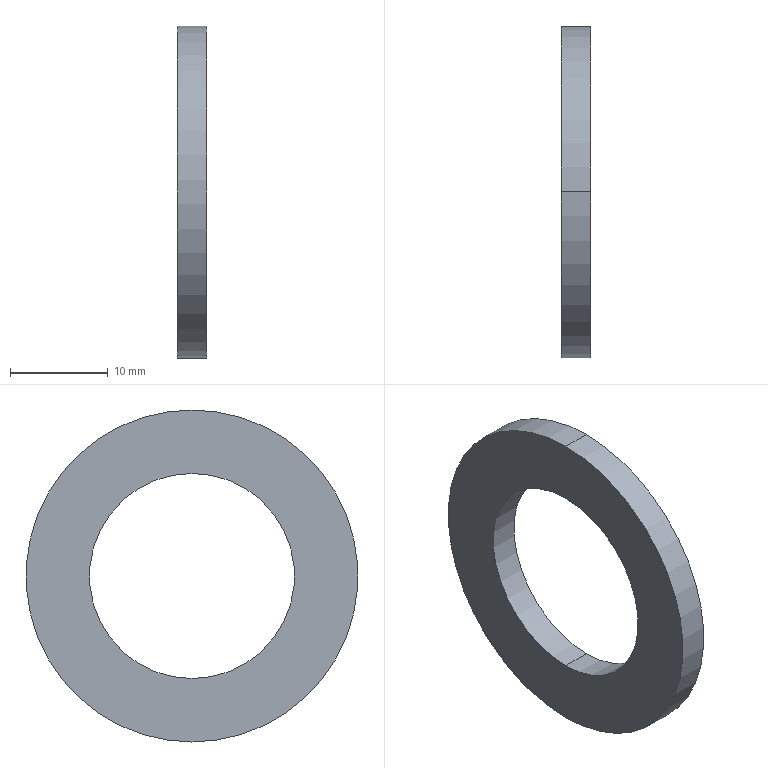Part | STEP file | plain washer small grade a_iso(Washer ISO 7092 - 20) | 1 solid | 6 faces | box 3 x 34 x 34 mm | volume 1685 mm3 | cylinder 4 | plane 2 | commonest cylinder face diameters 21 x2 34 x2
STEP:
#1=CARTESIAN_POINT('',(0.,0.,0.));
#2=DIRECTION('',(0.,0.,1.));
#3=DIRECTION('',(1.,0.,0.));
#4=AXIS2_PLACEMENT_3D('',#1,#2,#3);
#5=CARTESIAN_POINT('',(0.,0.,17.));
#6=VERTEX_POINT('',#5);
#7=CARTESIAN_POINT('',(0.,0.,-17.));
#8=VERTEX_POINT('',#7);
#9=CARTESIAN_POINT('',(0.,0.,0.));
#10=DIRECTION('',(-1.,0.,0.));
#11=DIRECTION('',(0.,0.,1.));
#12=AXIS2_PLACEMENT_3D('',#9,#10,#11);
#13=CIRCLE('',#12,17.);
#14=CARTESIAN_POINT('',(-34.925,0.,0.));
#15=DIRECTION('',(-1.,0.,0.));
#16=DIRECTION('',(0.,0.,1.));
#17=AXIS2_PLACEMENT_3D('',#14,#15,#16);
#18=CYLINDRICAL_SURFACE('',#17,17.);
#19=CARTESIAN_POINT('',(0.,-34.925));
#20=DIRECTION('',(1.,0.));
#21=VECTOR('',#20,1.);
#22=LINE('',#19,#21);
#23=(GEOMETRIC_REPRESENTATION_CONTEXT(2)PARAMETRIC_REPRESENTATION_CONTEXT()REPRESENTATION_CONTEXT('',''));
#24=DEFINITIONAL_REPRESENTATION('',(#22),#23);
#25=PCURVE('',#18,#24);
#26=CARTESIAN_POINT('',(0.,10.5,0.));
#27=DIRECTION('',(-1.,0.,0.));
#28=DIRECTION('',(0.,0.,1.));
#29=AXIS2_PLACEMENT_3D('',#26,#27,#28);
#30=PLANE('',#29);
#31=CARTESIAN_POINT('',(0.,-10.5));
#32=DIRECTION('',(1.,0.));
#33=AXIS2_PLACEMENT_2D('',#31,#32);
#34=CIRCLE('',#33,17.);
#35=(GEOMETRIC_REPRESENTATION_CONTEXT(2)PARAMETRIC_REPRESENTATION_CONTEXT()REPRESENTATION_CONTEXT('',''));
#36=DEFINITIONAL_REPRESENTATION('',(#34),#35);
#37=PCURVE('',#30,#36);
#38=SURFACE_CURVE('',#13,(#25,#37),.PCURVE_S1.);
#39=EDGE_CURVE('',#6,#8,#38,.T.);
#40=ORIENTED_EDGE('',*,*,#39,.T.);
#41=CARTESIAN_POINT('',(-3.,0.,-17.));
#42=VERTEX_POINT('',#41);
#43=CARTESIAN_POINT('',(-34.925,0.,-17.));
#44=DIRECTION('',(-1.,0.,0.));
#45=VECTOR('',#44,1.);
#46=LINE('',#43,#45);
#47=CARTESIAN_POINT('',(3.142,0.));
#48=DIRECTION('',(0.,1.));
#49=VECTOR('',#48,1.);
#50=LINE('',#47,#49);
#51=(GEOMETRIC_REPRESENTATION_CONTEXT(2)PARAMETRIC_REPRESENTATION_CONTEXT()REPRESENTATION_CONTEXT('',''));
#52=DEFINITIONAL_REPRESENTATION('',(#50),#51);
#53=PCURVE('',#18,#52);
#54=CARTESIAN_POINT('',(-34.925,0.,0.));
#55=DIRECTION('',(-1.,0.,0.));
#56=DIRECTION('',(0.,0.,1.));
#57=AXIS2_PLACEMENT_3D('',#54,#55,#56);
#58=CYLINDRICAL_SURFACE('',#57,17.);
#59=CARTESIAN_POINT('',(3.142,0.));
#60=DIRECTION('',(0.,1.));
#61=VECTOR('',#60,1.);
#62=LINE('',#59,#61);
#63=(GEOMETRIC_REPRESENTATION_CONTEXT(2)PARAMETRIC_REPRESENTATION_CONTEXT()REPRESENTATION_CONTEXT('',''));
#64=DEFINITIONAL_REPRESENTATION('',(#62),#63);
#65=PCURVE('',#58,#64);
#66=SURFACE_CURVE('',#46,(#53,#65),.PCURVE_S1.);
#67=EDGE_CURVE('',#8,#42,#66,.T.);
#68=ORIENTED_EDGE('',*,*,#67,.T.);
#69=CARTESIAN_POINT('',(-3.,0.,17.));
#70=VERTEX_POINT('',#69);
#71=CARTESIAN_POINT('',(-3.,0.,0.));
#72=DIRECTION('',(-1.,0.,0.));
#73=DIRECTION('',(0.,0.,1.));
#74=AXIS2_PLACEMENT_3D('',#71,#72,#73);
#75=CIRCLE('',#74,17.);
#76=CARTESIAN_POINT('',(0.,-31.925));
#77=DIRECTION('',(1.,0.));
#78=VECTOR('',#77,1.);
#79=LINE('',#76,#78);
#80=(GEOMETRIC_REPRESENTATION_CONTEXT(2)PARAMETRIC_REPRESENTATION_CONTEXT()REPRESENTATION_CONTEXT('',''));
#81=DEFINITIONAL_REPRESENTATION('',(#79),#80);
#82=PCURVE('',#18,#81);
#83=CARTESIAN_POINT('',(-3.,17.,0.));
#84=DIRECTION('',(1.,0.,0.));
#85=DIRECTION('',(0.,0.,-1.));
#86=AXIS2_PLACEMENT_3D('',#83,#84,#85);
#87=PLANE('',#86);
#88=CARTESIAN_POINT('',(-17.,-17.));
#89=CARTESIAN_POINT('',(-17.,12.445));
#90=CARTESIAN_POINT('',(8.5,-2.278));
#91=CARTESIAN_POINT('',(34.,-17.));
#92=CARTESIAN_POINT('',(8.5,-31.722));
#93=CARTESIAN_POINT('',(-17.,-46.445));
#94=CARTESIAN_POINT('',(-17.,-17.));
#95=(BOUNDED_CURVE()B_SPLINE_CURVE(2,(#88,#89,#90,#91,#92,#93,#94),.UNSPECIFIED.,.T.,.F.)B_SPLINE_CURVE_WITH_KNOTS((1,2,2,2,2,1),(-2.094,0.,2.094,4.189,6.283,8.378),.UNSPECIFIED.)CURVE()GEOMETRIC_REPRESENTATION_ITEM()RATIONAL_B_SPLINE_CURVE((1.,0.5,1.,0.5,1.,0.5,1.))REPRESENTATION_ITEM(''));
#96=(GEOMETRIC_REPRESENTATION_CONTEXT(2)PARAMETRIC_REPRESENTATION_CONTEXT()REPRESENTATION_CONTEXT('',''));
#97=DEFINITIONAL_REPRESENTATION('',(#95),#96);
#98=PCURVE('',#87,#97);
#99=SURFACE_CURVE('',#75,(#82,#98),.PCURVE_S1.);
#100=EDGE_CURVE('',#70,#42,#99,.T.);
#101=ORIENTED_EDGE('',*,*,#100,.F.);
#102=CARTESIAN_POINT('',(-34.925,0.,17.));
#103=DIRECTION('',(-1.,0.,0.));
#104=VECTOR('',#103,1.);
#105=LINE('',#102,#104);
#106=CARTESIAN_POINT('',(0.,0.));
#107=DIRECTION('',(0.,1.));
#108=VECTOR('',#107,1.);
#109=LINE('',#106,#108);
#110=(GEOMETRIC_REPRESENTATION_CONTEXT(2)PARAMETRIC_REPRESENTATION_CONTEXT()REPRESENTATION_CONTEXT('',''));
#111=DEFINITIONAL_REPRESENTATION('',(#109),#110);
#112=PCURVE('',#18,#111);
#113=CARTESIAN_POINT('',(6.283,0.));
#114=DIRECTION('',(0.,1.));
#115=VECTOR('',#114,1.);
#116=LINE('',#113,#115);
#117=(GEOMETRIC_REPRESENTATION_CONTEXT(2)PARAMETRIC_REPRESENTATION_CONTEXT()REPRESENTATION_CONTEXT('',''));
#118=DEFINITIONAL_REPRESENTATION('',(#116),#117);
#119=PCURVE('',#58,#118);
#120=SURFACE_CURVE('',#105,(#112,#119),.PCURVE_S1.);
#121=EDGE_CURVE('',#6,#70,#120,.T.);
#122=ORIENTED_EDGE('',*,*,#121,.F.);
#123=EDGE_LOOP('',(#40,#68,#101,#122));
#124=FACE_BOUND('',#123,.T.);
#125=ADVANCED_FACE('',(#124),#18,.T.);
#126=CARTESIAN_POINT('',(0.,0.,10.5));
#127=VERTEX_POINT('',#126);
#128=CARTESIAN_POINT('',(-3.,0.,10.5));
#129=VERTEX_POINT('',#128);
#130=CARTESIAN_POINT('',(-34.925,0.,10.5));
#131=DIRECTION('',(-1.,0.,0.));
#132=VECTOR('',#131,1.);
#133=LINE('',#130,#132);
#134=CARTESIAN_POINT('',(-34.925,0.,0.));
#135=DIRECTION('',(-1.,0.,0.));
#136=DIRECTION('',(0.,0.,1.));
#137=AXIS2_PLACEMENT_3D('',#134,#135,#136);
#138=CYLINDRICAL_SURFACE('',#137,10.5);
#139=CARTESIAN_POINT('',(6.283,0.));
#140=DIRECTION('',(0.,1.));
#141=VECTOR('',#140,1.);
#142=LINE('',#139,#141);
#143=(GEOMETRIC_REPRESENTATION_CONTEXT(2)PARAMETRIC_REPRESENTATION_CONTEXT()REPRESENTATION_CONTEXT('',''));
#144=DEFINITIONAL_REPRESENTATION('',(#142),#143);
#145=PCURVE('',#138,#144);
#146=CARTESIAN_POINT('',(-34.925,0.,0.));
#147=DIRECTION('',(-1.,0.,0.));
#148=DIRECTION('',(0.,0.,1.));
#149=AXIS2_PLACEMENT_3D('',#146,#147,#148);
#150=CYLINDRICAL_SURFACE('',#149,10.5);
#151=CARTESIAN_POINT('',(0.,0.));
#152=DIRECTION('',(0.,1.));
#153=VECTOR('',#152,1.);
#154=LINE('',#151,#153);
#155=(GEOMETRIC_REPRESENTATION_CONTEXT(2)PARAMETRIC_REPRESENTATION_CONTEXT()REPRESENTATION_CONTEXT('',''));
#156=DEFINITIONAL_REPRESENTATION('',(#154),#155);
#157=PCURVE('',#150,#156);
#158=SURFACE_CURVE('',#133,(#145,#157),.PCURVE_S1.);
#159=EDGE_CURVE('',#127,#129,#158,.T.);
#160=ORIENTED_EDGE('',*,*,#159,.T.);
#161=CARTESIAN_POINT('',(-3.,0.,-10.5));
#162=VERTEX_POINT('',#161);
#163=CARTESIAN_POINT('',(-3.,0.,0.));
#164=DIRECTION('',(-1.,0.,0.));
#165=DIRECTION('',(0.,0.,1.));
#166=AXIS2_PLACEMENT_3D('',#163,#164,#165);
#167=CIRCLE('',#166,10.5);
#168=CARTESIAN_POINT('',(0.,-31.925));
#169=DIRECTION('',(1.,0.));
#170=VECTOR('',#169,1.);
#171=LINE('',#168,#170);
#172=(GEOMETRIC_REPRESENTATION_CONTEXT(2)PARAMETRIC_REPRESENTATION_CONTEXT()REPRESENTATION_CONTEXT('',''));
#173=DEFINITIONAL_REPRESENTATION('',(#171),#172);
#174=PCURVE('',#138,#173);
#175=CARTESIAN_POINT('',(-10.5,-17.));
#176=CARTESIAN_POINT('',(-10.5,1.187));
#177=CARTESIAN_POINT('',(5.25,-7.907));
#178=CARTESIAN_POINT('',(21.,-17.));
#179=CARTESIAN_POINT('',(5.25,-26.093));
#180=CARTESIAN_POINT('',(-10.5,-35.187));
#181=CARTESIAN_POINT('',(-10.5,-17.));
#182=(BOUNDED_CURVE()B_SPLINE_CURVE(2,(#175,#176,#177,#178,#179,#180,#181),.UNSPECIFIED.,.T.,.F.)B_SPLINE_CURVE_WITH_KNOTS((1,2,2,2,2,1),(-2.094,0.,2.094,4.189,6.283,8.378),.UNSPECIFIED.)CURVE()GEOMETRIC_REPRESENTATION_ITEM()RATIONAL_B_SPLINE_CURVE((1.,0.5,1.,0.5,1.,0.5,1.))REPRESENTATION_ITEM(''));
#183=(GEOMETRIC_REPRESENTATION_CONTEXT(2)PARAMETRIC_REPRESENTATION_CONTEXT()REPRESENTATION_CONTEXT('',''));
#184=DEFINITIONAL_REPRESENTATION('',(#182),#183);
#185=PCURVE('',#87,#184);
#186=SURFACE_CURVE('',#167,(#174,#185),.PCURVE_S1.);
#187=EDGE_CURVE('',#162,#129,#186,.T.);
#188=ORIENTED_EDGE('',*,*,#187,.F.);
#189=CARTESIAN_POINT('',(0.,0.,-10.5));
#190=VERTEX_POINT('',#189);
#191=CARTESIAN_POINT('',(-34.925,0.,-10.5));
#192=DIRECTION('',(-1.,0.,0.));
#193=VECTOR('',#192,1.);
#194=LINE('',#191,#193);
#195=CARTESIAN_POINT('',(3.142,0.));
#196=DIRECTION('',(0.,1.));
#197=VECTOR('',#196,1.);
#198=LINE('',#195,#197);
#199=(GEOMETRIC_REPRESENTATION_CONTEXT(2)PARAMETRIC_REPRESENTATION_CONTEXT()REPRESENTATION_CONTEXT('',''));
#200=DEFINITIONAL_REPRESENTATION('',(#198),#199);
#201=PCURVE('',#138,#200);
#202=CARTESIAN_POINT('',(3.142,0.));
#203=DIRECTION('',(0.,1.));
#204=VECTOR('',#203,1.);
#205=LINE('',#202,#204);
#206=(GEOMETRIC_REPRESENTATION_CONTEXT(2)PARAMETRIC_REPRESENTATION_CONTEXT()REPRESENTATION_CONTEXT('',''));
#207=DEFINITIONAL_REPRESENTATION('',(#205),#206);
#208=PCURVE('',#150,#207);
#209=SURFACE_CURVE('',#194,(#201,#208),.PCURVE_S1.);
#210=EDGE_CURVE('',#190,#162,#209,.T.);
#211=ORIENTED_EDGE('',*,*,#210,.F.);
#212=CARTESIAN_POINT('',(0.,0.,0.));
#213=DIRECTION('',(-1.,0.,0.));
#214=DIRECTION('',(0.,0.,1.));
#215=AXIS2_PLACEMENT_3D('',#212,#213,#214);
#216=CIRCLE('',#215,10.5);
#217=CARTESIAN_POINT('',(0.,-34.925));
#218=DIRECTION('',(1.,0.));
#219=VECTOR('',#218,1.);
#220=LINE('',#217,#219);
#221=(GEOMETRIC_REPRESENTATION_CONTEXT(2)PARAMETRIC_REPRESENTATION_CONTEXT()REPRESENTATION_CONTEXT('',''));
#222=DEFINITIONAL_REPRESENTATION('',(#220),#221);
#223=PCURVE('',#138,#222);
#224=CARTESIAN_POINT('',(0.,-10.5));
#225=DIRECTION('',(1.,0.));
#226=AXIS2_PLACEMENT_2D('',#224,#225);
#227=CIRCLE('',#226,10.5);
#228=(GEOMETRIC_REPRESENTATION_CONTEXT(2)PARAMETRIC_REPRESENTATION_CONTEXT()REPRESENTATION_CONTEXT('',''));
#229=DEFINITIONAL_REPRESENTATION('',(#227),#228);
#230=PCURVE('',#30,#229);
#231=SURFACE_CURVE('',#216,(#223,#230),.PCURVE_S1.);
#232=EDGE_CURVE('',#190,#127,#231,.T.);
#233=ORIENTED_EDGE('',*,*,#232,.T.);
#234=EDGE_LOOP('',(#160,#188,#211,#233));
#235=FACE_BOUND('',#234,.F.);
#236=ADVANCED_FACE('',(#235),#138,.F.);
#237=CARTESIAN_POINT('',(-3.,0.,0.));
#238=DIRECTION('',(-1.,0.,0.));
#239=DIRECTION('',(0.,0.,1.));
#240=AXIS2_PLACEMENT_3D('',#237,#238,#239);
#241=CIRCLE('',#240,10.5);
#242=CARTESIAN_POINT('',(0.,-31.925));
#243=DIRECTION('',(1.,0.));
#244=VECTOR('',#243,1.);
#245=LINE('',#242,#244);
#246=(GEOMETRIC_REPRESENTATION_CONTEXT(2)PARAMETRIC_REPRESENTATION_CONTEXT()REPRESENTATION_CONTEXT('',''));
#247=DEFINITIONAL_REPRESENTATION('',(#245),#246);
#248=PCURVE('',#150,#247);
#249=CARTESIAN_POINT('',(-10.5,-17.));
#250=CARTESIAN_POINT('',(-10.5,1.187));
#251=CARTESIAN_POINT('',(5.25,-7.907));
#252=CARTESIAN_POINT('',(21.,-17.));
#253=CARTESIAN_POINT('',(5.25,-26.093));
#254=CARTESIAN_POINT('',(-10.5,-35.187));
#255=CARTESIAN_POINT('',(-10.5,-17.));
#256=(BOUNDED_CURVE()B_SPLINE_CURVE(2,(#249,#250,#251,#252,#253,#254,#255),.UNSPECIFIED.,.T.,.F.)B_SPLINE_CURVE_WITH_KNOTS((1,2,2,2,2,1),(-2.094,0.,2.094,4.189,6.283,8.378),.UNSPECIFIED.)CURVE()GEOMETRIC_REPRESENTATION_ITEM()RATIONAL_B_SPLINE_CURVE((1.,0.5,1.,0.5,1.,0.5,1.))REPRESENTATION_ITEM(''));
#257=(GEOMETRIC_REPRESENTATION_CONTEXT(2)PARAMETRIC_REPRESENTATION_CONTEXT()REPRESENTATION_CONTEXT('',''));
#258=DEFINITIONAL_REPRESENTATION('',(#256),#257);
#259=PCURVE('',#87,#258);
#260=SURFACE_CURVE('',#241,(#248,#259),.PCURVE_S1.);
#261=EDGE_CURVE('',#129,#162,#260,.T.);
#262=ORIENTED_EDGE('',*,*,#261,.F.);
#263=ORIENTED_EDGE('',*,*,#159,.F.);
#264=CARTESIAN_POINT('',(0.,0.,0.));
#265=DIRECTION('',(-1.,0.,0.));
#266=DIRECTION('',(0.,0.,1.));
#267=AXIS2_PLACEMENT_3D('',#264,#265,#266);
#268=CIRCLE('',#267,10.5);
#269=CARTESIAN_POINT('',(0.,-34.925));
#270=DIRECTION('',(1.,0.));
#271=VECTOR('',#270,1.);
#272=LINE('',#269,#271);
#273=(GEOMETRIC_REPRESENTATION_CONTEXT(2)PARAMETRIC_REPRESENTATION_CONTEXT()REPRESENTATION_CONTEXT('',''));
#274=DEFINITIONAL_REPRESENTATION('',(#272),#273);
#275=PCURVE('',#150,#274);
#276=CARTESIAN_POINT('',(0.,-10.5));
#277=DIRECTION('',(1.,0.));
#278=AXIS2_PLACEMENT_2D('',#276,#277);
#279=CIRCLE('',#278,10.5);
#280=(GEOMETRIC_REPRESENTATION_CONTEXT(2)PARAMETRIC_REPRESENTATION_CONTEXT()REPRESENTATION_CONTEXT('',''));
#281=DEFINITIONAL_REPRESENTATION('',(#279),#280);
#282=PCURVE('',#30,#281);
#283=SURFACE_CURVE('',#268,(#275,#282),.PCURVE_S1.);
#284=EDGE_CURVE('',#127,#190,#283,.T.);
#285=ORIENTED_EDGE('',*,*,#284,.T.);
#286=ORIENTED_EDGE('',*,*,#210,.T.);
#287=EDGE_LOOP('',(#262,#263,#285,#286));
#288=FACE_BOUND('',#287,.F.);
#289=ADVANCED_FACE('',(#288),#150,.F.);
#290=ORIENTED_EDGE('',*,*,#39,.F.);
#291=CARTESIAN_POINT('',(0.,0.,0.));
#292=DIRECTION('',(-1.,0.,0.));
#293=DIRECTION('',(0.,0.,1.));
#294=AXIS2_PLACEMENT_3D('',#291,#292,#293);
#295=CIRCLE('',#294,17.);
#296=CARTESIAN_POINT('',(0.,-10.5));
#297=DIRECTION('',(1.,0.));
#298=AXIS2_PLACEMENT_2D('',#296,#297);
#299=CIRCLE('',#298,17.);
#300=(GEOMETRIC_REPRESENTATION_CONTEXT(2)PARAMETRIC_REPRESENTATION_CONTEXT()REPRESENTATION_CONTEXT('',''));
#301=DEFINITIONAL_REPRESENTATION('',(#299),#300);
#302=PCURVE('',#30,#301);
#303=CARTESIAN_POINT('',(0.,-34.925));
#304=DIRECTION('',(1.,0.));
#305=VECTOR('',#304,1.);
#306=LINE('',#303,#305);
#307=(GEOMETRIC_REPRESENTATION_CONTEXT(2)PARAMETRIC_REPRESENTATION_CONTEXT()REPRESENTATION_CONTEXT('',''));
#308=DEFINITIONAL_REPRESENTATION('',(#306),#307);
#309=PCURVE('',#58,#308);
#310=SURFACE_CURVE('',#295,(#302,#309),.PCURVE_S1.);
#311=EDGE_CURVE('',#8,#6,#310,.T.);
#312=ORIENTED_EDGE('',*,*,#311,.F.);
#313=EDGE_LOOP('',(#290,#312));
#314=FACE_BOUND('',#313,.T.);
#315=ORIENTED_EDGE('',*,*,#284,.T.);
#316=ORIENTED_EDGE('',*,*,#232,.T.);
#317=EDGE_LOOP('',(#315,#316));
#318=FACE_BOUND('',#317,.T.);
#319=ADVANCED_FACE('',(#314,#318),#30,.F.);
#320=ORIENTED_EDGE('',*,*,#67,.F.);
#321=ORIENTED_EDGE('',*,*,#311,.T.);
#322=ORIENTED_EDGE('',*,*,#121,.T.);
#323=CARTESIAN_POINT('',(-3.,0.,0.));
#324=DIRECTION('',(-1.,0.,0.));
#325=DIRECTION('',(0.,0.,1.));
#326=AXIS2_PLACEMENT_3D('',#323,#324,#325);
#327=CIRCLE('',#326,17.);
#328=CARTESIAN_POINT('',(0.,-31.925));
#329=DIRECTION('',(1.,0.));
#330=VECTOR('',#329,1.);
#331=LINE('',#328,#330);
#332=(GEOMETRIC_REPRESENTATION_CONTEXT(2)PARAMETRIC_REPRESENTATION_CONTEXT()REPRESENTATION_CONTEXT('',''));
#333=DEFINITIONAL_REPRESENTATION('',(#331),#332);
#334=PCURVE('',#58,#333);
#335=CARTESIAN_POINT('',(-17.,-17.));
#336=CARTESIAN_POINT('',(-17.,12.445));
#337=CARTESIAN_POINT('',(8.5,-2.278));
#338=CARTESIAN_POINT('',(34.,-17.));
#339=CARTESIAN_POINT('',(8.5,-31.722));
#340=CARTESIAN_POINT('',(-17.,-46.445));
#341=CARTESIAN_POINT('',(-17.,-17.));
#342=(BOUNDED_CURVE()B_SPLINE_CURVE(2,(#335,#336,#337,#338,#339,#340,#341),.UNSPECIFIED.,.T.,.F.)B_SPLINE_CURVE_WITH_KNOTS((1,2,2,2,2,1),(-2.094,0.,2.094,4.189,6.283,8.378),.UNSPECIFIED.)CURVE()GEOMETRIC_REPRESENTATION_ITEM()RATIONAL_B_SPLINE_CURVE((1.,0.5,1.,0.5,1.,0.5,1.))REPRESENTATION_ITEM(''));
#343=(GEOMETRIC_REPRESENTATION_CONTEXT(2)PARAMETRIC_REPRESENTATION_CONTEXT()REPRESENTATION_CONTEXT('',''));
#344=DEFINITIONAL_REPRESENTATION('',(#342),#343);
#345=PCURVE('',#87,#344);
#346=SURFACE_CURVE('',#327,(#334,#345),.PCURVE_S1.);
#347=EDGE_CURVE('',#42,#70,#346,.T.);
#348=ORIENTED_EDGE('',*,*,#347,.F.);
#349=EDGE_LOOP('',(#320,#321,#322,#348));
#350=FACE_BOUND('',#349,.T.);
#351=ADVANCED_FACE('',(#350),#58,.T.);
#352=ORIENTED_EDGE('',*,*,#261,.F.);
#353=ORIENTED_EDGE('',*,*,#187,.F.);
#354=EDGE_LOOP('',(#352,#353));
#355=FACE_BOUND('',#354,.T.);
#356=ORIENTED_EDGE('',*,*,#100,.T.);
#357=ORIENTED_EDGE('',*,*,#347,.T.);
#358=EDGE_LOOP('',(#356,#357));
#359=FACE_BOUND('',#358,.T.);
#360=ADVANCED_FACE('',(#355,#359),#87,.F.);
#361=CLOSED_SHELL('',(#125,#236,#289,#319,#351,#360));
#362=MANIFOLD_SOLID_BREP('',#361);
#363=(LENGTH_UNIT()NAMED_UNIT(*)SI_UNIT(.MILLI.,.METRE.));
#364=UNCERTAINTY_MEASURE_WITH_UNIT(LENGTH_MEASURE(0.0000001),#363,'','');
#365=(NAMED_UNIT(*)PLANE_ANGLE_UNIT()SI_UNIT($,.RADIAN.));
#366=(NAMED_UNIT(*)SI_UNIT($,.STERADIAN.)SOLID_ANGLE_UNIT());
#367=(GEOMETRIC_REPRESENTATION_CONTEXT(3)GLOBAL_UNCERTAINTY_ASSIGNED_CONTEXT((#364))GLOBAL_UNIT_ASSIGNED_CONTEXT((#363,#365,#366))REPRESENTATION_CONTEXT('',''));
#368=ADVANCED_BREP_SHAPE_REPRESENTATION('',(#4,#362),#367);